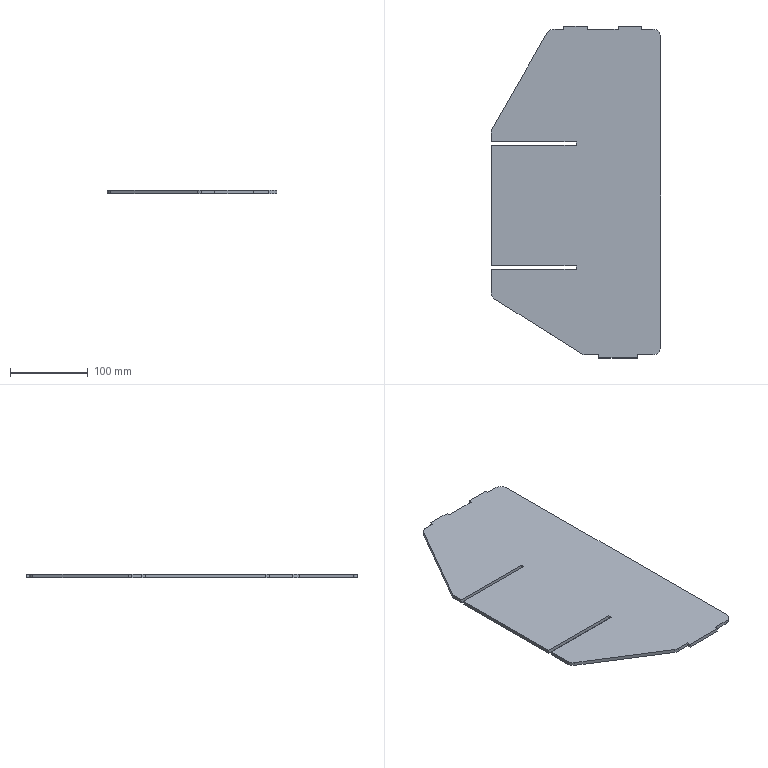Part | SolidWorks | features FlatPattern 1, SMBaseFlange 1, SheetMetal 1 | 1 solid | 34 faces | box 218.7 x 428.4 x 4.5 mm | volume 369053 mm3 | plane 28 | cylinder 6 | commonest cylinder face diameters 20 x6
STEP:
#1=CARTESIAN_POINT('',(-227.2,-382.479,0.));
#2=VERTEX_POINT('',#1);
#3=CARTESIAN_POINT('',(-227.2,-395.3,0.));
#4=VERTEX_POINT('',#3);
#5=CARTESIAN_POINT('',(-227.2,-395.3,0.));
#6=DIRECTION('',(0.,-1.,0.));
#7=VECTOR('',#6,1000.);
#8=LINE('',#5,#7);
#9=EDGE_CURVE('',#2,#4,#8,.T.);
#10=ORIENTED_EDGE('',*,*,#9,.T.);
#11=CARTESIAN_POINT('',(-227.2,-395.3,4.5));
#12=VERTEX_POINT('',#11);
#13=CARTESIAN_POINT('',(-227.2,-395.3,4.5));
#14=DIRECTION('',(0.,0.,-1.));
#15=VECTOR('',#14,1000.);
#16=LINE('',#13,#15);
#17=EDGE_CURVE('',#12,#4,#16,.T.);
#18=ORIENTED_EDGE('',*,*,#17,.F.);
#19=CARTESIAN_POINT('',(-227.2,-382.479,4.5));
#20=VERTEX_POINT('',#19);
#21=CARTESIAN_POINT('',(-227.2,-395.3,4.5));
#22=DIRECTION('',(0.,-1.,0.));
#23=VECTOR('',#22,1000.);
#24=LINE('',#21,#23);
#25=EDGE_CURVE('',#20,#12,#24,.T.);
#26=ORIENTED_EDGE('',*,*,#25,.F.);
#27=CARTESIAN_POINT('',(-227.2,-382.479,4.5));
#28=DIRECTION('',(0.,0.,-1.));
#29=VECTOR('',#28,1000.);
#30=LINE('',#27,#29);
#31=EDGE_CURVE('',#20,#2,#30,.T.);
#32=ORIENTED_EDGE('',*,*,#31,.T.);
#33=EDGE_LOOP('',(#10,#18,#26,#32));
#34=FACE_OUTER_BOUND('',#33,.T.);
#35=CARTESIAN_POINT('',(-227.2,-395.3,4.5));
#36=DIRECTION('',(1.,0.,0.));
#37=DIRECTION('',(0.,0.,-1.));
#38=AXIS2_PLACEMENT_3D('',#35,#36,#37);
#39=PLANE('',#38);
#40=ADVANCED_FACE('',(#34),#39,.F.);
#41=CARTESIAN_POINT('',(-117.7,-395.3,0.));
#42=VERTEX_POINT('',#41);
#43=CARTESIAN_POINT('',(-227.2,-395.3,0.));
#44=DIRECTION('',(1.,0.,0.));
#45=VECTOR('',#44,1000.);
#46=LINE('',#43,#45);
#47=EDGE_CURVE('',#4,#42,#46,.T.);
#48=ORIENTED_EDGE('',*,*,#47,.T.);
#49=CARTESIAN_POINT('',(-117.7,-395.3,4.5));
#50=VERTEX_POINT('',#49);
#51=CARTESIAN_POINT('',(-117.7,-395.3,4.5));
#52=DIRECTION('',(0.,0.,-1.));
#53=VECTOR('',#52,1000.);
#54=LINE('',#51,#53);
#55=EDGE_CURVE('',#50,#42,#54,.T.);
#56=ORIENTED_EDGE('',*,*,#55,.F.);
#57=CARTESIAN_POINT('',(-227.2,-395.3,4.5));
#58=DIRECTION('',(1.,0.,0.));
#59=VECTOR('',#58,1000.);
#60=LINE('',#57,#59);
#61=EDGE_CURVE('',#12,#50,#60,.T.);
#62=ORIENTED_EDGE('',*,*,#61,.F.);
#63=ORIENTED_EDGE('',*,*,#17,.T.);
#64=EDGE_LOOP('',(#48,#56,#62,#63));
#65=FACE_OUTER_BOUND('',#64,.T.);
#66=CARTESIAN_POINT('',(-227.2,-395.3,4.5));
#67=DIRECTION('',(0.,1.,0.));
#68=DIRECTION('',(-1.,0.,0.));
#69=AXIS2_PLACEMENT_3D('',#66,#67,#68);
#70=PLANE('',#69);
#71=ADVANCED_FACE('',(#65),#70,.F.);
#72=CARTESIAN_POINT('',(-117.7,-399.8,0.));
#73=VERTEX_POINT('',#72);
#74=CARTESIAN_POINT('',(-117.7,-395.3,0.));
#75=DIRECTION('',(0.,-1.,0.));
#76=VECTOR('',#75,1000.);
#77=LINE('',#74,#76);
#78=EDGE_CURVE('',#42,#73,#77,.T.);
#79=ORIENTED_EDGE('',*,*,#78,.T.);
#80=CARTESIAN_POINT('',(-117.7,-399.8,4.5));
#81=VERTEX_POINT('',#80);
#82=CARTESIAN_POINT('',(-117.7,-399.8,4.5));
#83=DIRECTION('',(0.,0.,-1.));
#84=VECTOR('',#83,1000.);
#85=LINE('',#82,#84);
#86=EDGE_CURVE('',#81,#73,#85,.T.);
#87=ORIENTED_EDGE('',*,*,#86,.F.);
#88=CARTESIAN_POINT('',(-117.7,-395.3,4.5));
#89=DIRECTION('',(0.,-1.,0.));
#90=VECTOR('',#89,1000.);
#91=LINE('',#88,#90);
#92=EDGE_CURVE('',#50,#81,#91,.T.);
#93=ORIENTED_EDGE('',*,*,#92,.F.);
#94=ORIENTED_EDGE('',*,*,#55,.T.);
#95=EDGE_LOOP('',(#79,#87,#93,#94));
#96=FACE_OUTER_BOUND('',#95,.T.);
#97=CARTESIAN_POINT('',(-117.7,-395.3,4.5));
#98=DIRECTION('',(1.,0.,0.));
#99=DIRECTION('',(0.,0.,-1.));
#100=AXIS2_PLACEMENT_3D('',#97,#98,#99);
#101=PLANE('',#100);
#102=ADVANCED_FACE('',(#96),#101,.F.);
#103=CARTESIAN_POINT('',(-227.2,-399.8,0.));
#104=VERTEX_POINT('',#103);
#105=CARTESIAN_POINT('',(-117.7,-399.8,0.));
#106=DIRECTION('',(-1.,0.,0.));
#107=VECTOR('',#106,1000.);
#108=LINE('',#105,#107);
#109=EDGE_CURVE('',#73,#104,#108,.T.);
#110=ORIENTED_EDGE('',*,*,#109,.T.);
#111=CARTESIAN_POINT('',(-227.2,-399.8,4.5));
#112=VERTEX_POINT('',#111);
#113=CARTESIAN_POINT('',(-227.2,-399.8,4.5));
#114=DIRECTION('',(0.,0.,-1.));
#115=VECTOR('',#114,1000.);
#116=LINE('',#113,#115);
#117=EDGE_CURVE('',#112,#104,#116,.T.);
#118=ORIENTED_EDGE('',*,*,#117,.F.);
#119=CARTESIAN_POINT('',(-117.7,-399.8,4.5));
#120=DIRECTION('',(-1.,0.,0.));
#121=VECTOR('',#120,1000.);
#122=LINE('',#119,#121);
#123=EDGE_CURVE('',#81,#112,#122,.T.);
#124=ORIENTED_EDGE('',*,*,#123,.F.);
#125=ORIENTED_EDGE('',*,*,#86,.T.);
#126=EDGE_LOOP('',(#110,#118,#124,#125));
#127=FACE_OUTER_BOUND('',#126,.T.);
#128=CARTESIAN_POINT('',(-117.7,-399.8,4.5));
#129=DIRECTION('',(0.,-1.,0.));
#130=DIRECTION('',(0.,0.,-1.));
#131=AXIS2_PLACEMENT_3D('',#128,#129,#130);
#132=PLANE('',#131);
#133=ADVANCED_FACE('',(#127),#132,.F.);
#134=CARTESIAN_POINT('',(-227.2,-555.3,0.));
#135=VERTEX_POINT('',#134);
#136=CARTESIAN_POINT('',(-227.2,-555.3,0.));
#137=DIRECTION('',(0.,-1.,0.));
#138=VECTOR('',#137,1000.);
#139=LINE('',#136,#138);
#140=EDGE_CURVE('',#104,#135,#139,.T.);
#141=ORIENTED_EDGE('',*,*,#140,.T.);
#142=CARTESIAN_POINT('',(-227.2,-555.3,4.5));
#143=VERTEX_POINT('',#142);
#144=CARTESIAN_POINT('',(-227.2,-555.3,4.5));
#145=DIRECTION('',(0.,0.,-1.));
#146=VECTOR('',#145,1000.);
#147=LINE('',#144,#146);
#148=EDGE_CURVE('',#143,#135,#147,.T.);
#149=ORIENTED_EDGE('',*,*,#148,.F.);
#150=CARTESIAN_POINT('',(-227.2,-555.3,4.5));
#151=DIRECTION('',(0.,-1.,0.));
#152=VECTOR('',#151,1000.);
#153=LINE('',#150,#152);
#154=EDGE_CURVE('',#112,#143,#153,.T.);
#155=ORIENTED_EDGE('',*,*,#154,.F.);
#156=ORIENTED_EDGE('',*,*,#117,.T.);
#157=EDGE_LOOP('',(#141,#149,#155,#156));
#158=FACE_OUTER_BOUND('',#157,.T.);
#159=CARTESIAN_POINT('',(-227.2,-555.3,4.5));
#160=DIRECTION('',(1.,0.,0.));
#161=DIRECTION('',(0.,0.,-1.));
#162=AXIS2_PLACEMENT_3D('',#159,#160,#161);
#163=PLANE('',#162);
#164=ADVANCED_FACE('',(#158),#163,.F.);
#165=CARTESIAN_POINT('',(-117.7,-555.3,0.));
#166=VERTEX_POINT('',#165);
#167=CARTESIAN_POINT('',(-227.2,-555.3,0.));
#168=DIRECTION('',(1.,0.,0.));
#169=VECTOR('',#168,1000.);
#170=LINE('',#167,#169);
#171=EDGE_CURVE('',#135,#166,#170,.T.);
#172=ORIENTED_EDGE('',*,*,#171,.T.);
#173=CARTESIAN_POINT('',(-117.7,-555.3,4.5));
#174=VERTEX_POINT('',#173);
#175=CARTESIAN_POINT('',(-117.7,-555.3,4.5));
#176=DIRECTION('',(0.,0.,-1.));
#177=VECTOR('',#176,1000.);
#178=LINE('',#175,#177);
#179=EDGE_CURVE('',#174,#166,#178,.T.);
#180=ORIENTED_EDGE('',*,*,#179,.F.);
#181=CARTESIAN_POINT('',(-227.2,-555.3,4.5));
#182=DIRECTION('',(1.,0.,0.));
#183=VECTOR('',#182,1000.);
#184=LINE('',#181,#183);
#185=EDGE_CURVE('',#143,#174,#184,.T.);
#186=ORIENTED_EDGE('',*,*,#185,.F.);
#187=ORIENTED_EDGE('',*,*,#148,.T.);
#188=EDGE_LOOP('',(#172,#180,#186,#187));
#189=FACE_OUTER_BOUND('',#188,.T.);
#190=CARTESIAN_POINT('',(-227.2,-555.3,4.5));
#191=DIRECTION('',(0.,1.,0.));
#192=DIRECTION('',(-1.,0.,0.));
#193=AXIS2_PLACEMENT_3D('',#190,#191,#192);
#194=PLANE('',#193);
#195=ADVANCED_FACE('',(#189),#194,.F.);
#196=CARTESIAN_POINT('',(-117.7,-559.8,0.));
#197=VERTEX_POINT('',#196);
#198=CARTESIAN_POINT('',(-117.7,-555.3,0.));
#199=DIRECTION('',(0.,-1.,0.));
#200=VECTOR('',#199,1000.);
#201=LINE('',#198,#200);
#202=EDGE_CURVE('',#166,#197,#201,.T.);
#203=ORIENTED_EDGE('',*,*,#202,.T.);
#204=CARTESIAN_POINT('',(-117.7,-559.8,4.5));
#205=VERTEX_POINT('',#204);
#206=CARTESIAN_POINT('',(-117.7,-559.8,4.5));
#207=DIRECTION('',(0.,0.,-1.));
#208=VECTOR('',#207,1000.);
#209=LINE('',#206,#208);
#210=EDGE_CURVE('',#205,#197,#209,.T.);
#211=ORIENTED_EDGE('',*,*,#210,.F.);
#212=CARTESIAN_POINT('',(-117.7,-555.3,4.5));
#213=DIRECTION('',(0.,-1.,0.));
#214=VECTOR('',#213,1000.);
#215=LINE('',#212,#214);
#216=EDGE_CURVE('',#174,#205,#215,.T.);
#217=ORIENTED_EDGE('',*,*,#216,.F.);
#218=ORIENTED_EDGE('',*,*,#179,.T.);
#219=EDGE_LOOP('',(#203,#211,#217,#218));
#220=FACE_OUTER_BOUND('',#219,.T.);
#221=CARTESIAN_POINT('',(-117.7,-555.3,4.5));
#222=DIRECTION('',(1.,0.,0.));
#223=DIRECTION('',(0.,1.,0.));
#224=AXIS2_PLACEMENT_3D('',#221,#222,#223);
#225=PLANE('',#224);
#226=ADVANCED_FACE('',(#220),#225,.F.);
#227=CARTESIAN_POINT('',(-227.2,-559.8,0.));
#228=VERTEX_POINT('',#227);
#229=CARTESIAN_POINT('',(-117.7,-559.8,0.));
#230=DIRECTION('',(-1.,0.,0.));
#231=VECTOR('',#230,1000.);
#232=LINE('',#229,#231);
#233=EDGE_CURVE('',#197,#228,#232,.T.);
#234=ORIENTED_EDGE('',*,*,#233,.T.);
#235=CARTESIAN_POINT('',(-227.2,-559.8,4.5));
#236=VERTEX_POINT('',#235);
#237=CARTESIAN_POINT('',(-227.2,-559.8,4.5));
#238=DIRECTION('',(0.,0.,-1.));
#239=VECTOR('',#238,1000.);
#240=LINE('',#237,#239);
#241=EDGE_CURVE('',#236,#228,#240,.T.);
#242=ORIENTED_EDGE('',*,*,#241,.F.);
#243=CARTESIAN_POINT('',(-117.7,-559.8,4.5));
#244=DIRECTION('',(-1.,0.,0.));
#245=VECTOR('',#244,1000.);
#246=LINE('',#243,#245);
#247=EDGE_CURVE('',#205,#236,#246,.T.);
#248=ORIENTED_EDGE('',*,*,#247,.F.);
#249=ORIENTED_EDGE('',*,*,#210,.T.);
#250=EDGE_LOOP('',(#234,#242,#248,#249));
#251=FACE_OUTER_BOUND('',#250,.T.);
#252=CARTESIAN_POINT('',(-117.7,-559.8,4.5));
#253=DIRECTION('',(0.,-1.,0.));
#254=DIRECTION('',(0.,0.,-1.));
#255=AXIS2_PLACEMENT_3D('',#252,#253,#254);
#256=PLANE('',#255);
#257=ADVANCED_FACE('',(#251),#256,.F.);
#258=CARTESIAN_POINT('',(-227.2,-589.69,0.));
#259=VERTEX_POINT('',#258);
#260=CARTESIAN_POINT('',(-227.2,-589.69,0.));
#261=DIRECTION('',(0.,-1.,0.));
#262=VECTOR('',#261,1000.);
#263=LINE('',#260,#262);
#264=EDGE_CURVE('',#228,#259,#263,.T.);
#265=ORIENTED_EDGE('',*,*,#264,.T.);
#266=CARTESIAN_POINT('',(-227.2,-589.69,4.5));
#267=VERTEX_POINT('',#266);
#268=CARTESIAN_POINT('',(-227.2,-589.69,4.5));
#269=DIRECTION('',(0.,0.,-1.));
#270=VECTOR('',#269,1000.);
#271=LINE('',#268,#270);
#272=EDGE_CURVE('',#267,#259,#271,.T.);
#273=ORIENTED_EDGE('',*,*,#272,.F.);
#274=CARTESIAN_POINT('',(-227.2,-589.69,4.5));
#275=DIRECTION('',(0.,-1.,0.));
#276=VECTOR('',#275,1000.);
#277=LINE('',#274,#276);
#278=EDGE_CURVE('',#236,#267,#277,.T.);
#279=ORIENTED_EDGE('',*,*,#278,.F.);
#280=ORIENTED_EDGE('',*,*,#241,.T.);
#281=EDGE_LOOP('',(#265,#273,#279,#280));
#282=FACE_OUTER_BOUND('',#281,.T.);
#283=CARTESIAN_POINT('',(-227.2,-589.69,4.5));
#284=DIRECTION('',(1.,0.,0.));
#285=DIRECTION('',(0.,0.,-1.));
#286=AXIS2_PLACEMENT_3D('',#283,#284,#285);
#287=PLANE('',#286);
#288=ADVANCED_FACE('',(#282),#287,.F.);
#289=CARTESIAN_POINT('',(-222.541,-598.143,0.));
#290=VERTEX_POINT('',#289);
#291=CARTESIAN_POINT('',(-217.2,-589.69,0.));
#292=DIRECTION('',(0.,0.,1.));
#293=DIRECTION('',(-1.,0.,0.));
#294=AXIS2_PLACEMENT_3D('',#291,#292,#293);
#295=CIRCLE('',#294,10.);
#296=EDGE_CURVE('',#259,#290,#295,.T.);
#297=ORIENTED_EDGE('',*,*,#296,.T.);
#298=CARTESIAN_POINT('',(-222.541,-598.143,4.5));
#299=VERTEX_POINT('',#298);
#300=CARTESIAN_POINT('',(-222.541,-598.143,4.5));
#301=DIRECTION('',(0.,0.,-1.));
#302=VECTOR('',#301,1000.);
#303=LINE('',#300,#302);
#304=EDGE_CURVE('',#299,#290,#303,.T.);
#305=ORIENTED_EDGE('',*,*,#304,.F.);
#306=CARTESIAN_POINT('',(-217.2,-589.69,4.5));
#307=DIRECTION('',(0.,0.,1.));
#308=DIRECTION('',(-1.,0.,0.));
#309=AXIS2_PLACEMENT_3D('',#306,#307,#308);
#310=CIRCLE('',#309,10.);
#311=EDGE_CURVE('',#267,#299,#310,.T.);
#312=ORIENTED_EDGE('',*,*,#311,.F.);
#313=ORIENTED_EDGE('',*,*,#272,.T.);
#314=EDGE_LOOP('',(#297,#305,#312,#313));
#315=FACE_OUTER_BOUND('',#314,.T.);
#316=CARTESIAN_POINT('',(-217.2,-589.69,4.5));
#317=DIRECTION('',(0.,0.,-1.));
#318=DIRECTION('',(-1.,0.,0.));
#319=AXIS2_PLACEMENT_3D('',#316,#317,#318);
#320=CYLINDRICAL_SURFACE('',#319,10.);
#321=ADVANCED_FACE('',(#315),#320,.T.);
#322=CARTESIAN_POINT('',(-110.947,-668.654,0.));
#323=VERTEX_POINT('',#322);
#324=CARTESIAN_POINT('',(-222.541,-598.143,0.));
#325=DIRECTION('',(0.8454,-0.5342,0.));
#326=VECTOR('',#325,1000.);
#327=LINE('',#324,#326);
#328=EDGE_CURVE('',#290,#323,#327,.T.);
#329=ORIENTED_EDGE('',*,*,#328,.T.);
#330=CARTESIAN_POINT('',(-110.947,-668.654,4.5));
#331=VERTEX_POINT('',#330);
#332=CARTESIAN_POINT('',(-110.947,-668.654,4.5));
#333=DIRECTION('',(0.,0.,-1.));
#334=VECTOR('',#333,1000.);
#335=LINE('',#332,#334);
#336=EDGE_CURVE('',#331,#323,#335,.T.);
#337=ORIENTED_EDGE('',*,*,#336,.F.);
#338=CARTESIAN_POINT('',(-222.541,-598.143,4.5));
#339=DIRECTION('',(0.8454,-0.5342,0.));
#340=VECTOR('',#339,1000.);
#341=LINE('',#338,#340);
#342=EDGE_CURVE('',#299,#331,#341,.T.);
#343=ORIENTED_EDGE('',*,*,#342,.F.);
#344=ORIENTED_EDGE('',*,*,#304,.T.);
#345=EDGE_LOOP('',(#329,#337,#343,#344));
#346=FACE_OUTER_BOUND('',#345,.T.);
#347=CARTESIAN_POINT('',(-222.541,-598.143,4.5));
#348=DIRECTION('',(0.5342,0.8454,0.));
#349=DIRECTION('',(-0.8454,0.5342,0.));
#350=AXIS2_PLACEMENT_3D('',#347,#348,#349);
#351=PLANE('',#350);
#352=ADVANCED_FACE('',(#346),#351,.F.);
#353=CARTESIAN_POINT('',(-105.605,-670.2,0.));
#354=VERTEX_POINT('',#353);
#355=CARTESIAN_POINT('',(-105.605,-660.2,0.));
#356=DIRECTION('',(0.,0.,1.));
#357=DIRECTION('',(-1.,0.,0.));
#358=AXIS2_PLACEMENT_3D('',#355,#356,#357);
#359=CIRCLE('',#358,10.);
#360=EDGE_CURVE('',#323,#354,#359,.T.);
#361=ORIENTED_EDGE('',*,*,#360,.T.);
#362=CARTESIAN_POINT('',(-105.605,-670.2,4.5));
#363=VERTEX_POINT('',#362);
#364=CARTESIAN_POINT('',(-105.605,-670.2,4.5));
#365=DIRECTION('',(0.,0.,-1.));
#366=VECTOR('',#365,1000.);
#367=LINE('',#364,#366);
#368=EDGE_CURVE('',#363,#354,#367,.T.);
#369=ORIENTED_EDGE('',*,*,#368,.F.);
#370=CARTESIAN_POINT('',(-105.605,-660.2,4.5));
#371=DIRECTION('',(0.,0.,1.));
#372=DIRECTION('',(-1.,0.,0.));
#373=AXIS2_PLACEMENT_3D('',#370,#371,#372);
#374=CIRCLE('',#373,10.);
#375=EDGE_CURVE('',#331,#363,#374,.T.);
#376=ORIENTED_EDGE('',*,*,#375,.F.);
#377=ORIENTED_EDGE('',*,*,#336,.T.);
#378=EDGE_LOOP('',(#361,#369,#376,#377));
#379=FACE_OUTER_BOUND('',#378,.T.);
#380=CARTESIAN_POINT('',(-105.605,-660.2,4.5));
#381=DIRECTION('',(0.,0.,-1.));
#382=DIRECTION('',(-1.,0.,0.));
#383=AXIS2_PLACEMENT_3D('',#380,#381,#382);
#384=CYLINDRICAL_SURFACE('',#383,10.);
#385=ADVANCED_FACE('',(#379),#384,.T.);
#386=CARTESIAN_POINT('',(-88.5,-670.2,0.));
#387=VERTEX_POINT('',#386);
#388=CARTESIAN_POINT('',(-105.605,-670.2,0.));
#389=DIRECTION('',(1.,0.,0.));
#390=VECTOR('',#389,1000.);
#391=LINE('',#388,#390);
#392=EDGE_CURVE('',#354,#387,#391,.T.);
#393=ORIENTED_EDGE('',*,*,#392,.T.);
#394=CARTESIAN_POINT('',(-88.5,-670.2,4.5));
#395=VERTEX_POINT('',#394);
#396=CARTESIAN_POINT('',(-88.5,-670.2,4.5));
#397=DIRECTION('',(0.,0.,-1.));
#398=VECTOR('',#397,1000.);
#399=LINE('',#396,#398);
#400=EDGE_CURVE('',#395,#387,#399,.T.);
#401=ORIENTED_EDGE('',*,*,#400,.F.);
#402=CARTESIAN_POINT('',(-105.605,-670.2,4.5));
#403=DIRECTION('',(1.,0.,0.));
#404=VECTOR('',#403,1000.);
#405=LINE('',#402,#404);
#406=EDGE_CURVE('',#363,#395,#405,.T.);
#407=ORIENTED_EDGE('',*,*,#406,.F.);
#408=ORIENTED_EDGE('',*,*,#368,.T.);
#409=EDGE_LOOP('',(#393,#401,#407,#408));
#410=FACE_OUTER_BOUND('',#409,.T.);
#411=CARTESIAN_POINT('',(-105.605,-670.2,4.5));
#412=DIRECTION('',(0.,1.,0.));
#413=DIRECTION('',(-1.,0.,0.));
#414=AXIS2_PLACEMENT_3D('',#411,#412,#413);
#415=PLANE('',#414);
#416=ADVANCED_FACE('',(#410),#415,.F.);
#417=CARTESIAN_POINT('',(-88.5,-674.2,0.));
#418=VERTEX_POINT('',#417);
#419=CARTESIAN_POINT('',(-88.5,-674.2,0.));
#420=DIRECTION('',(0.,-1.,0.));
#421=VECTOR('',#420,1000.);
#422=LINE('',#419,#421);
#423=EDGE_CURVE('',#387,#418,#422,.T.);
#424=ORIENTED_EDGE('',*,*,#423,.T.);
#425=CARTESIAN_POINT('',(-88.5,-674.2,4.5));
#426=VERTEX_POINT('',#425);
#427=CARTESIAN_POINT('',(-88.5,-674.2,4.5));
#428=DIRECTION('',(0.,0.,-1.));
#429=VECTOR('',#428,1000.);
#430=LINE('',#427,#429);
#431=EDGE_CURVE('',#426,#418,#430,.T.);
#432=ORIENTED_EDGE('',*,*,#431,.F.);
#433=CARTESIAN_POINT('',(-88.5,-674.2,4.5));
#434=DIRECTION('',(0.,-1.,0.));
#435=VECTOR('',#434,1000.);
#436=LINE('',#433,#435);
#437=EDGE_CURVE('',#395,#426,#436,.T.);
#438=ORIENTED_EDGE('',*,*,#437,.F.);
#439=ORIENTED_EDGE('',*,*,#400,.T.);
#440=EDGE_LOOP('',(#424,#432,#438,#439));
#441=FACE_OUTER_BOUND('',#440,.T.);
#442=CARTESIAN_POINT('',(-88.5,-674.2,4.5));
#443=DIRECTION('',(1.,0.,0.));
#444=DIRECTION('',(0.,0.,-1.));
#445=AXIS2_PLACEMENT_3D('',#442,#443,#444);
#446=PLANE('',#445);
#447=ADVANCED_FACE('',(#441),#446,.F.);
#448=CARTESIAN_POINT('',(-38.5,-674.2,0.));
#449=VERTEX_POINT('',#448);
#450=CARTESIAN_POINT('',(-38.5,-674.2,0.));
#451=DIRECTION('',(1.,0.,0.));
#452=VECTOR('',#451,1000.);
#453=LINE('',#450,#452);
#454=EDGE_CURVE('',#418,#449,#453,.T.);
#455=ORIENTED_EDGE('',*,*,#454,.T.);
#456=CARTESIAN_POINT('',(-38.5,-674.2,4.5));
#457=VERTEX_POINT('',#456);
#458=CARTESIAN_POINT('',(-38.5,-674.2,4.5));
#459=DIRECTION('',(0.,0.,-1.));
#460=VECTOR('',#459,1000.);
#461=LINE('',#458,#460);
#462=EDGE_CURVE('',#457,#449,#461,.T.);
#463=ORIENTED_EDGE('',*,*,#462,.F.);
#464=CARTESIAN_POINT('',(-38.5,-674.2,4.5));
#465=DIRECTION('',(1.,0.,0.));
#466=VECTOR('',#465,1000.);
#467=LINE('',#464,#466);
#468=EDGE_CURVE('',#426,#457,#467,.T.);
#469=ORIENTED_EDGE('',*,*,#468,.F.);
#470=ORIENTED_EDGE('',*,*,#431,.T.);
#471=EDGE_LOOP('',(#455,#463,#469,#470));
#472=FACE_OUTER_BOUND('',#471,.T.);
#473=CARTESIAN_POINT('',(-38.5,-674.2,4.5));
#474=DIRECTION('',(0.,1.,0.));
#475=DIRECTION('',(0.,0.,1.));
#476=AXIS2_PLACEMENT_3D('',#473,#474,#475);
#477=PLANE('',#476);
#478=ADVANCED_FACE('',(#472),#477,.F.);
#479=CARTESIAN_POINT('',(-38.5,-670.2,0.));
#480=VERTEX_POINT('',#479);
#481=CARTESIAN_POINT('',(-38.5,-670.2,0.));
#482=DIRECTION('',(0.,1.,0.));
#483=VECTOR('',#482,1000.);
#484=LINE('',#481,#483);
#485=EDGE_CURVE('',#449,#480,#484,.T.);
#486=ORIENTED_EDGE('',*,*,#485,.T.);
#487=CARTESIAN_POINT('',(-38.5,-670.2,4.5));
#488=VERTEX_POINT('',#487);
#489=CARTESIAN_POINT('',(-38.5,-670.2,4.5));
#490=DIRECTION('',(0.,0.,-1.));
#491=VECTOR('',#490,1000.);
#492=LINE('',#489,#491);
#493=EDGE_CURVE('',#488,#480,#492,.T.);
#494=ORIENTED_EDGE('',*,*,#493,.F.);
#495=CARTESIAN_POINT('',(-38.5,-670.2,4.5));
#496=DIRECTION('',(0.,1.,0.));
#497=VECTOR('',#496,1000.);
#498=LINE('',#495,#497);
#499=EDGE_CURVE('',#457,#488,#498,.T.);
#500=ORIENTED_EDGE('',*,*,#499,.F.);
#501=ORIENTED_EDGE('',*,*,#462,.T.);
#502=EDGE_LOOP('',(#486,#494,#500,#501));
#503=FACE_OUTER_BOUND('',#502,.T.);
#504=CARTESIAN_POINT('',(-38.5,-670.2,4.5));
#505=DIRECTION('',(-1.,0.,0.));
#506=DIRECTION('',(0.,-1.,0.));
#507=AXIS2_PLACEMENT_3D('',#504,#505,#506);
#508=PLANE('',#507);
#509=ADVANCED_FACE('',(#503),#508,.F.);
#510=CARTESIAN_POINT('',(-18.5,-670.2,0.));
#511=VERTEX_POINT('',#510);
#512=CARTESIAN_POINT('',(-18.5,-670.2,0.));
#513=DIRECTION('',(1.,0.,0.));
#514=VECTOR('',#513,1000.);
#515=LINE('',#512,#514);
#516=EDGE_CURVE('',#480,#511,#515,.T.);
#517=ORIENTED_EDGE('',*,*,#516,.T.);
#518=CARTESIAN_POINT('',(-18.5,-670.2,4.5));
#519=VERTEX_POINT('',#518);
#520=CARTESIAN_POINT('',(-18.5,-670.2,4.5));
#521=DIRECTION('',(0.,0.,-1.));
#522=VECTOR('',#521,1000.);
#523=LINE('',#520,#522);
#524=EDGE_CURVE('',#519,#511,#523,.T.);
#525=ORIENTED_EDGE('',*,*,#524,.F.);
#526=CARTESIAN_POINT('',(-18.5,-670.2,4.5));
#527=DIRECTION('',(1.,0.,0.));
#528=VECTOR('',#527,1000.);
#529=LINE('',#526,#528);
#530=EDGE_CURVE('',#488,#519,#529,.T.);
#531=ORIENTED_EDGE('',*,*,#530,.F.);
#532=ORIENTED_EDGE('',*,*,#493,.T.);
#533=EDGE_LOOP('',(#517,#525,#531,#532));
#534=FACE_OUTER_BOUND('',#533,.T.);
#535=CARTESIAN_POINT('',(-18.5,-670.2,4.5));
#536=DIRECTION('',(0.,1.,0.));
#537=DIRECTION('',(-1.,0.,0.));
#538=AXIS2_PLACEMENT_3D('',#535,#536,#537);
#539=PLANE('',#538);
#540=ADVANCED_FACE('',(#534),#539,.F.);
#541=CARTESIAN_POINT('',(-8.5,-660.2,0.));
#542=VERTEX_POINT('',#541);
#543=CARTESIAN_POINT('',(-18.5,-660.2,0.));
#544=DIRECTION('',(0.,0.,1.));
#545=DIRECTION('',(-1.,0.,0.));
#546=AXIS2_PLACEMENT_3D('',#543,#544,#545);
#547=CIRCLE('',#546,10.);
#548=EDGE_CURVE('',#511,#542,#547,.T.);
#549=ORIENTED_EDGE('',*,*,#548,.T.);
#550=CARTESIAN_POINT('',(-8.5,-660.2,4.5));
#551=VERTEX_POINT('',#550);
#552=CARTESIAN_POINT('',(-8.5,-660.2,4.5));
#553=DIRECTION('',(0.,0.,-1.));
#554=VECTOR('',#553,1000.);
#555=LINE('',#552,#554);
#556=EDGE_CURVE('',#551,#542,#555,.T.);
#557=ORIENTED_EDGE('',*,*,#556,.F.);
#558=CARTESIAN_POINT('',(-18.5,-660.2,4.5));
#559=DIRECTION('',(0.,0.,1.));
#560=DIRECTION('',(-1.,0.,0.));
#561=AXIS2_PLACEMENT_3D('',#558,#559,#560);
#562=CIRCLE('',#561,10.);
#563=EDGE_CURVE('',#519,#551,#562,.T.);
#564=ORIENTED_EDGE('',*,*,#563,.F.);
#565=ORIENTED_EDGE('',*,*,#524,.T.);
#566=EDGE_LOOP('',(#549,#557,#564,#565));
#567=FACE_OUTER_BOUND('',#566,.T.);
#568=CARTESIAN_POINT('',(-18.5,-660.2,4.5));
#569=DIRECTION('',(0.,0.,-1.));
#570=DIRECTION('',(-1.,0.,0.));
#571=AXIS2_PLACEMENT_3D('',#568,#569,#570);
#572=CYLINDRICAL_SURFACE('',#571,10.);
#573=ADVANCED_FACE('',(#567),#572,.T.);
#574=CARTESIAN_POINT('',(-8.5,-259.8,0.));
#575=VERTEX_POINT('',#574);
#576=CARTESIAN_POINT('',(-8.5,-259.8,0.));
#577=DIRECTION('',(0.,1.,0.));
#578=VECTOR('',#577,1000.);
#579=LINE('',#576,#578);
#580=EDGE_CURVE('',#542,#575,#579,.T.);
#581=ORIENTED_EDGE('',*,*,#580,.T.);
#582=CARTESIAN_POINT('',(-8.5,-259.8,4.5));
#583=VERTEX_POINT('',#582);
#584=CARTESIAN_POINT('',(-8.5,-259.8,4.5));
#585=DIRECTION('',(0.,0.,-1.));
#586=VECTOR('',#585,1000.);
#587=LINE('',#584,#586);
#588=EDGE_CURVE('',#583,#575,#587,.T.);
#589=ORIENTED_EDGE('',*,*,#588,.F.);
#590=CARTESIAN_POINT('',(-8.5,-259.8,4.5));
#591=DIRECTION('',(0.,1.,0.));
#592=VECTOR('',#591,1000.);
#593=LINE('',#590,#592);
#594=EDGE_CURVE('',#551,#583,#593,.T.);
#595=ORIENTED_EDGE('',*,*,#594,.F.);
#596=ORIENTED_EDGE('',*,*,#556,.T.);
#597=EDGE_LOOP('',(#581,#589,#595,#596));
#598=FACE_OUTER_BOUND('',#597,.T.);
#599=CARTESIAN_POINT('',(-8.5,-259.8,4.5));
#600=DIRECTION('',(-1.,0.,0.));
#601=DIRECTION('',(0.,-1.,0.));
#602=AXIS2_PLACEMENT_3D('',#599,#600,#601);
#603=PLANE('',#602);
#604=ADVANCED_FACE('',(#598),#603,.F.);
#605=CARTESIAN_POINT('',(-18.5,-249.8,0.));
#606=VERTEX_POINT('',#605);
#607=CARTESIAN_POINT('',(-18.5,-259.8,0.));
#608=DIRECTION('',(0.,0.,1.));
#609=DIRECTION('',(1.,0.,0.));
#610=AXIS2_PLACEMENT_3D('',#607,#608,#609);
#611=CIRCLE('',#610,10.);
#612=EDGE_CURVE('',#575,#606,#611,.T.);
#613=ORIENTED_EDGE('',*,*,#612,.T.);
#614=CARTESIAN_POINT('',(-18.5,-249.8,4.5));
#615=VERTEX_POINT('',#614);
#616=CARTESIAN_POINT('',(-18.5,-249.8,4.5));
#617=DIRECTION('',(0.,0.,-1.));
#618=VECTOR('',#617,1000.);
#619=LINE('',#616,#618);
#620=EDGE_CURVE('',#615,#606,#619,.T.);
#621=ORIENTED_EDGE('',*,*,#620,.F.);
#622=CARTESIAN_POINT('',(-18.5,-259.8,4.5));
#623=DIRECTION('',(0.,0.,1.));
#624=DIRECTION('',(1.,0.,0.));
#625=AXIS2_PLACEMENT_3D('',#622,#623,#624);
#626=CIRCLE('',#625,10.);
#627=EDGE_CURVE('',#583,#615,#626,.T.);
#628=ORIENTED_EDGE('',*,*,#627,.F.);
#629=ORIENTED_EDGE('',*,*,#588,.T.);
#630=EDGE_LOOP('',(#613,#621,#628,#629));
#631=FACE_OUTER_BOUND('',#630,.T.);
#632=CARTESIAN_POINT('',(-18.5,-259.8,4.5));
#633=DIRECTION('',(0.,0.,-1.));
#634=DIRECTION('',(-1.,0.,0.));
#635=AXIS2_PLACEMENT_3D('',#632,#633,#634);
#636=CYLINDRICAL_SURFACE('',#635,10.);
#637=ADVANCED_FACE('',(#631),#636,.T.);
#638=CARTESIAN_POINT('',(-33.5,-249.8,0.));
#639=VERTEX_POINT('',#638);
#640=CARTESIAN_POINT('',(-18.5,-249.8,0.));
#641=DIRECTION('',(-1.,0.,0.));
#642=VECTOR('',#641,1000.);
#643=LINE('',#640,#642);
#644=EDGE_CURVE('',#606,#639,#643,.T.);
#645=ORIENTED_EDGE('',*,*,#644,.T.);
#646=CARTESIAN_POINT('',(-33.5,-249.8,4.5));
#647=VERTEX_POINT('',#646);
#648=CARTESIAN_POINT('',(-33.5,-249.8,4.5));
#649=DIRECTION('',(0.,0.,-1.));
#650=VECTOR('',#649,1000.);
#651=LINE('',#648,#650);
#652=EDGE_CURVE('',#647,#639,#651,.T.);
#653=ORIENTED_EDGE('',*,*,#652,.F.);
#654=CARTESIAN_POINT('',(-18.5,-249.8,4.5));
#655=DIRECTION('',(-1.,0.,0.));
#656=VECTOR('',#655,1000.);
#657=LINE('',#654,#656);
#658=EDGE_CURVE('',#615,#647,#657,.T.);
#659=ORIENTED_EDGE('',*,*,#658,.F.);
#660=ORIENTED_EDGE('',*,*,#620,.T.);
#661=EDGE_LOOP('',(#645,#653,#659,#660));
#662=FACE_OUTER_BOUND('',#661,.T.);
#663=CARTESIAN_POINT('',(-18.5,-249.8,4.5));
#664=DIRECTION('',(0.,-1.,0.));
#665=DIRECTION('',(1.,0.,0.));
#666=AXIS2_PLACEMENT_3D('',#663,#664,#665);
#667=PLANE('',#666);
#668=ADVANCED_FACE('',(#662),#667,.F.);
#669=CARTESIAN_POINT('',(-33.5,-245.8,0.));
#670=VERTEX_POINT('',#669);
#671=CARTESIAN_POINT('',(-33.5,-249.8,0.));
#672=DIRECTION('',(0.,1.,0.));
#673=VECTOR('',#672,1000.);
#674=LINE('',#671,#673);
#675=EDGE_CURVE('',#639,#670,#674,.T.);
#676=ORIENTED_EDGE('',*,*,#675,.T.);
#677=CARTESIAN_POINT('',(-33.5,-245.8,4.5));
#678=VERTEX_POINT('',#677);
#679=CARTESIAN_POINT('',(-33.5,-245.8,4.5));
#680=DIRECTION('',(0.,0.,-1.));
#681=VECTOR('',#680,1000.);
#682=LINE('',#679,#681);
#683=EDGE_CURVE('',#678,#670,#682,.T.);
#684=ORIENTED_EDGE('',*,*,#683,.F.);
#685=CARTESIAN_POINT('',(-33.5,-249.8,4.5));
#686=DIRECTION('',(0.,1.,0.));
#687=VECTOR('',#686,1000.);
#688=LINE('',#685,#687);
#689=EDGE_CURVE('',#647,#678,#688,.T.);
#690=ORIENTED_EDGE('',*,*,#689,.F.);
#691=ORIENTED_EDGE('',*,*,#652,.T.);
#692=EDGE_LOOP('',(#676,#684,#690,#691));
#693=FACE_OUTER_BOUND('',#692,.T.);
#694=CARTESIAN_POINT('',(-33.5,-249.8,4.5));
#695=DIRECTION('',(-1.,0.,0.));
#696=DIRECTION('',(0.,0.,1.));
#697=AXIS2_PLACEMENT_3D('',#694,#695,#696);
#698=PLANE('',#697);
#699=ADVANCED_FACE('',(#693),#698,.F.);
#700=CARTESIAN_POINT('',(-63.5,-245.8,0.));
#701=VERTEX_POINT('',#700);
#702=CARTESIAN_POINT('',(-33.5,-245.8,0.));
#703=DIRECTION('',(-1.,0.,0.));
#704=VECTOR('',#703,1000.);
#705=LINE('',#702,#704);
#706=EDGE_CURVE('',#670,#701,#705,.T.);
#707=ORIENTED_EDGE('',*,*,#706,.T.);
#708=CARTESIAN_POINT('',(-63.5,-245.8,4.5));
#709=VERTEX_POINT('',#708);
#710=CARTESIAN_POINT('',(-63.5,-245.8,4.5));
#711=DIRECTION('',(0.,0.,-1.));
#712=VECTOR('',#711,1000.);
#713=LINE('',#710,#712);
#714=EDGE_CURVE('',#709,#701,#713,.T.);
#715=ORIENTED_EDGE('',*,*,#714,.F.);
#716=CARTESIAN_POINT('',(-33.5,-245.8,4.5));
#717=DIRECTION('',(-1.,0.,0.));
#718=VECTOR('',#717,1000.);
#719=LINE('',#716,#718);
#720=EDGE_CURVE('',#678,#709,#719,.T.);
#721=ORIENTED_EDGE('',*,*,#720,.F.);
#722=ORIENTED_EDGE('',*,*,#683,.T.);
#723=EDGE_LOOP('',(#707,#715,#721,#722));
#724=FACE_OUTER_BOUND('',#723,.T.);
#725=CARTESIAN_POINT('',(-33.5,-245.8,4.5));
#726=DIRECTION('',(0.,-1.,0.));
#727=DIRECTION('',(0.,0.,-1.));
#728=AXIS2_PLACEMENT_3D('',#725,#726,#727);
#729=PLANE('',#728);
#730=ADVANCED_FACE('',(#724),#729,.F.);
#731=CARTESIAN_POINT('',(-63.5,-249.8,0.));
#732=VERTEX_POINT('',#731);
#733=CARTESIAN_POINT('',(-63.5,-245.8,0.));
#734=DIRECTION('',(0.,-1.,0.));
#735=VECTOR('',#734,1000.);
#736=LINE('',#733,#735);
#737=EDGE_CURVE('',#701,#732,#736,.T.);
#738=ORIENTED_EDGE('',*,*,#737,.T.);
#739=CARTESIAN_POINT('',(-63.5,-249.8,4.5));
#740=VERTEX_POINT('',#739);
#741=CARTESIAN_POINT('',(-63.5,-249.8,4.5));
#742=DIRECTION('',(0.,0.,-1.));
#743=VECTOR('',#742,1000.);
#744=LINE('',#741,#743);
#745=EDGE_CURVE('',#740,#732,#744,.T.);
#746=ORIENTED_EDGE('',*,*,#745,.F.);
#747=CARTESIAN_POINT('',(-63.5,-245.8,4.5));
#748=DIRECTION('',(0.,-1.,0.));
#749=VECTOR('',#748,1000.);
#750=LINE('',#747,#749);
#751=EDGE_CURVE('',#709,#740,#750,.T.);
#752=ORIENTED_EDGE('',*,*,#751,.F.);
#753=ORIENTED_EDGE('',*,*,#714,.T.);
#754=EDGE_LOOP('',(#738,#746,#752,#753));
#755=FACE_OUTER_BOUND('',#754,.T.);
#756=CARTESIAN_POINT('',(-63.5,-245.8,4.5));
#757=DIRECTION('',(1.,0.,0.));
#758=DIRECTION('',(0.,0.,-1.));
#759=AXIS2_PLACEMENT_3D('',#756,#757,#758);
#760=PLANE('',#759);
#761=ADVANCED_FACE('',(#755),#760,.F.);
#762=CARTESIAN_POINT('',(-103.5,-249.8,0.));
#763=VERTEX_POINT('',#762);
#764=CARTESIAN_POINT('',(-63.5,-249.8,0.));
#765=DIRECTION('',(-1.,0.,0.));
#766=VECTOR('',#765,1000.);
#767=LINE('',#764,#766);
#768=EDGE_CURVE('',#732,#763,#767,.T.);
#769=ORIENTED_EDGE('',*,*,#768,.T.);
#770=CARTESIAN_POINT('',(-103.5,-249.8,4.5));
#771=VERTEX_POINT('',#770);
#772=CARTESIAN_POINT('',(-103.5,-249.8,4.5));
#773=DIRECTION('',(0.,0.,-1.));
#774=VECTOR('',#773,1000.);
#775=LINE('',#772,#774);
#776=EDGE_CURVE('',#771,#763,#775,.T.);
#777=ORIENTED_EDGE('',*,*,#776,.F.);
#778=CARTESIAN_POINT('',(-63.5,-249.8,4.5));
#779=DIRECTION('',(-1.,0.,0.));
#780=VECTOR('',#779,1000.);
#781=LINE('',#778,#780);
#782=EDGE_CURVE('',#740,#771,#781,.T.);
#783=ORIENTED_EDGE('',*,*,#782,.F.);
#784=ORIENTED_EDGE('',*,*,#745,.T.);
#785=EDGE_LOOP('',(#769,#777,#783,#784));
#786=FACE_OUTER_BOUND('',#785,.T.);
#787=CARTESIAN_POINT('',(-63.5,-249.8,4.5));
#788=DIRECTION('',(0.,-1.,0.));
#789=DIRECTION('',(0.,0.,-1.));
#790=AXIS2_PLACEMENT_3D('',#787,#788,#789);
#791=PLANE('',#790);
#792=ADVANCED_FACE('',(#786),#791,.F.);
#793=CARTESIAN_POINT('',(-103.5,-245.8,0.));
#794=VERTEX_POINT('',#793);
#795=CARTESIAN_POINT('',(-103.5,-249.8,0.));
#796=DIRECTION('',(0.,1.,0.));
#797=VECTOR('',#796,1000.);
#798=LINE('',#795,#797);
#799=EDGE_CURVE('',#763,#794,#798,.T.);
#800=ORIENTED_EDGE('',*,*,#799,.T.);
#801=CARTESIAN_POINT('',(-103.5,-245.8,4.5));
#802=VERTEX_POINT('',#801);
#803=CARTESIAN_POINT('',(-103.5,-245.8,4.5));
#804=DIRECTION('',(0.,0.,-1.));
#805=VECTOR('',#804,1000.);
#806=LINE('',#803,#805);
#807=EDGE_CURVE('',#802,#794,#806,.T.);
#808=ORIENTED_EDGE('',*,*,#807,.F.);
#809=CARTESIAN_POINT('',(-103.5,-249.8,4.5));
#810=DIRECTION('',(0.,1.,0.));
#811=VECTOR('',#810,1000.);
#812=LINE('',#809,#811);
#813=EDGE_CURVE('',#771,#802,#812,.T.);
#814=ORIENTED_EDGE('',*,*,#813,.F.);
#815=ORIENTED_EDGE('',*,*,#776,.T.);
#816=EDGE_LOOP('',(#800,#808,#814,#815));
#817=FACE_OUTER_BOUND('',#816,.T.);
#818=CARTESIAN_POINT('',(-103.5,-249.8,4.5));
#819=DIRECTION('',(-1.,0.,0.));
#820=DIRECTION('',(0.,0.,1.));
#821=AXIS2_PLACEMENT_3D('',#818,#819,#820);
#822=PLANE('',#821);
#823=ADVANCED_FACE('',(#817),#822,.F.);
#824=CARTESIAN_POINT('',(-133.5,-245.8,0.));
#825=VERTEX_POINT('',#824);
#826=CARTESIAN_POINT('',(-103.5,-245.8,0.));
#827=DIRECTION('',(-1.,0.,0.));
#828=VECTOR('',#827,1000.);
#829=LINE('',#826,#828);
#830=EDGE_CURVE('',#794,#825,#829,.T.);
#831=ORIENTED_EDGE('',*,*,#830,.T.);
#832=CARTESIAN_POINT('',(-133.5,-245.8,4.5));
#833=VERTEX_POINT('',#832);
#834=CARTESIAN_POINT('',(-133.5,-245.8,4.5));
#835=DIRECTION('',(0.,0.,-1.));
#836=VECTOR('',#835,1000.);
#837=LINE('',#834,#836);
#838=EDGE_CURVE('',#833,#825,#837,.T.);
#839=ORIENTED_EDGE('',*,*,#838,.F.);
#840=CARTESIAN_POINT('',(-103.5,-245.8,4.5));
#841=DIRECTION('',(-1.,0.,0.));
#842=VECTOR('',#841,1000.);
#843=LINE('',#840,#842);
#844=EDGE_CURVE('',#802,#833,#843,.T.);
#845=ORIENTED_EDGE('',*,*,#844,.F.);
#846=ORIENTED_EDGE('',*,*,#807,.T.);
#847=EDGE_LOOP('',(#831,#839,#845,#846));
#848=FACE_OUTER_BOUND('',#847,.T.);
#849=CARTESIAN_POINT('',(-103.5,-245.8,4.5));
#850=DIRECTION('',(0.,-1.,0.));
#851=DIRECTION('',(1.,0.,0.));
#852=AXIS2_PLACEMENT_3D('',#849,#850,#851);
#853=PLANE('',#852);
#854=ADVANCED_FACE('',(#848),#853,.F.);
#855=CARTESIAN_POINT('',(-133.5,-249.8,0.));
#856=VERTEX_POINT('',#855);
#857=CARTESIAN_POINT('',(-133.5,-245.8,0.));
#858=DIRECTION('',(0.,-1.,0.));
#859=VECTOR('',#858,1000.);
#860=LINE('',#857,#859);
#861=EDGE_CURVE('',#825,#856,#860,.T.);
#862=ORIENTED_EDGE('',*,*,#861,.T.);
#863=CARTESIAN_POINT('',(-133.5,-249.8,4.5));
#864=VERTEX_POINT('',#863);
#865=CARTESIAN_POINT('',(-133.5,-249.8,4.5));
#866=DIRECTION('',(0.,0.,-1.));
#867=VECTOR('',#866,1000.);
#868=LINE('',#865,#867);
#869=EDGE_CURVE('',#864,#856,#868,.T.);
#870=ORIENTED_EDGE('',*,*,#869,.F.);
#871=CARTESIAN_POINT('',(-133.5,-245.8,4.5));
#872=DIRECTION('',(0.,-1.,0.));
#873=VECTOR('',#872,1000.);
#874=LINE('',#871,#873);
#875=EDGE_CURVE('',#833,#864,#874,.T.);
#876=ORIENTED_EDGE('',*,*,#875,.F.);
#877=ORIENTED_EDGE('',*,*,#838,.T.);
#878=EDGE_LOOP('',(#862,#870,#876,#877));
#879=FACE_OUTER_BOUND('',#878,.T.);
#880=CARTESIAN_POINT('',(-133.5,-245.8,4.5));
#881=DIRECTION('',(1.,0.,0.));
#882=DIRECTION('',(0.,0.,-1.));
#883=AXIS2_PLACEMENT_3D('',#880,#881,#882);
#884=PLANE('',#883);
#885=ADVANCED_FACE('',(#879),#884,.F.);
#886=CARTESIAN_POINT('',(-146.371,-249.8,0.));
#887=VERTEX_POINT('',#886);
#888=CARTESIAN_POINT('',(-133.5,-249.8,0.));
#889=DIRECTION('',(-1.,0.,0.));
#890=VECTOR('',#889,1000.);
#891=LINE('',#888,#890);
#892=EDGE_CURVE('',#856,#887,#891,.T.);
#893=ORIENTED_EDGE('',*,*,#892,.T.);
#894=CARTESIAN_POINT('',(-146.371,-249.8,4.5));
#895=VERTEX_POINT('',#894);
#896=CARTESIAN_POINT('',(-146.371,-249.8,4.5));
#897=DIRECTION('',(0.,0.,-1.));
#898=VECTOR('',#897,1000.);
#899=LINE('',#896,#898);
#900=EDGE_CURVE('',#895,#887,#899,.T.);
#901=ORIENTED_EDGE('',*,*,#900,.F.);
#902=CARTESIAN_POINT('',(-133.5,-249.8,4.5));
#903=DIRECTION('',(-1.,0.,0.));
#904=VECTOR('',#903,1000.);
#905=LINE('',#902,#904);
#906=EDGE_CURVE('',#864,#895,#905,.T.);
#907=ORIENTED_EDGE('',*,*,#906,.F.);
#908=ORIENTED_EDGE('',*,*,#869,.T.);
#909=EDGE_LOOP('',(#893,#901,#907,#908));
#910=FACE_OUTER_BOUND('',#909,.T.);
#911=CARTESIAN_POINT('',(-133.5,-249.8,4.5));
#912=DIRECTION('',(0.,-1.,0.));
#913=DIRECTION('',(1.,0.,0.));
#914=AXIS2_PLACEMENT_3D('',#911,#912,#913);
#915=PLANE('',#914);
#916=ADVANCED_FACE('',(#910),#915,.F.);
#917=CARTESIAN_POINT('',(-155.031,-254.8,0.));
#918=VERTEX_POINT('',#917);
#919=CARTESIAN_POINT('',(-146.371,-259.8,0.));
#920=DIRECTION('',(0.,0.,1.));
#921=DIRECTION('',(1.,0.,0.));
#922=AXIS2_PLACEMENT_3D('',#919,#920,#921);
#923=CIRCLE('',#922,10.);
#924=EDGE_CURVE('',#887,#918,#923,.T.);
#925=ORIENTED_EDGE('',*,*,#924,.T.);
#926=CARTESIAN_POINT('',(-155.031,-254.8,4.5));
#927=VERTEX_POINT('',#926);
#928=CARTESIAN_POINT('',(-155.031,-254.8,4.5));
#929=DIRECTION('',(0.,0.,-1.));
#930=VECTOR('',#929,1000.);
#931=LINE('',#928,#930);
#932=EDGE_CURVE('',#927,#918,#931,.T.);
#933=ORIENTED_EDGE('',*,*,#932,.F.);
#934=CARTESIAN_POINT('',(-146.371,-259.8,4.5));
#935=DIRECTION('',(0.,0.,1.));
#936=DIRECTION('',(1.,0.,0.));
#937=AXIS2_PLACEMENT_3D('',#934,#935,#936);
#938=CIRCLE('',#937,10.);
#939=EDGE_CURVE('',#895,#927,#938,.T.);
#940=ORIENTED_EDGE('',*,*,#939,.F.);
#941=ORIENTED_EDGE('',*,*,#900,.T.);
#942=EDGE_LOOP('',(#925,#933,#940,#941));
#943=FACE_OUTER_BOUND('',#942,.T.);
#944=CARTESIAN_POINT('',(-146.371,-259.8,4.5));
#945=DIRECTION('',(0.,0.,-1.));
#946=DIRECTION('',(-1.,0.,0.));
#947=AXIS2_PLACEMENT_3D('',#944,#945,#946);
#948=CYLINDRICAL_SURFACE('',#947,10.);
#949=ADVANCED_FACE('',(#943),#948,.T.);
#950=CARTESIAN_POINT('',(-225.86,-377.479,0.));
#951=VERTEX_POINT('',#950);
#952=CARTESIAN_POINT('',(-225.86,-377.479,0.));
#953=DIRECTION('',(-0.5,-0.866,0.));
#954=VECTOR('',#953,1000.);
#955=LINE('',#952,#954);
#956=EDGE_CURVE('',#918,#951,#955,.T.);
#957=ORIENTED_EDGE('',*,*,#956,.T.);
#958=CARTESIAN_POINT('',(-225.86,-377.479,4.5));
#959=VERTEX_POINT('',#958);
#960=CARTESIAN_POINT('',(-225.86,-377.479,4.5));
#961=DIRECTION('',(0.,0.,-1.));
#962=VECTOR('',#961,1000.);
#963=LINE('',#960,#962);
#964=EDGE_CURVE('',#959,#951,#963,.T.);
#965=ORIENTED_EDGE('',*,*,#964,.F.);
#966=CARTESIAN_POINT('',(-225.86,-377.479,4.5));
#967=DIRECTION('',(-0.5,-0.866,0.));
#968=VECTOR('',#967,1000.);
#969=LINE('',#966,#968);
#970=EDGE_CURVE('',#927,#959,#969,.T.);
#971=ORIENTED_EDGE('',*,*,#970,.F.);
#972=ORIENTED_EDGE('',*,*,#932,.T.);
#973=EDGE_LOOP('',(#957,#965,#971,#972));
#974=FACE_OUTER_BOUND('',#973,.T.);
#975=CARTESIAN_POINT('',(-225.86,-377.479,4.5));
#976=DIRECTION('',(0.866,-0.5,0.));
#977=DIRECTION('',(0.5,0.866,0.));
#978=AXIS2_PLACEMENT_3D('',#975,#976,#977);
#979=PLANE('',#978);
#980=ADVANCED_FACE('',(#974),#979,.F.);
#981=CARTESIAN_POINT('',(-217.2,-382.479,0.));
#982=DIRECTION('',(0.,0.,1.));
#983=DIRECTION('',(-1.,0.,0.));
#984=AXIS2_PLACEMENT_3D('',#981,#982,#983);
#985=CIRCLE('',#984,10.);
#986=EDGE_CURVE('',#951,#2,#985,.T.);
#987=ORIENTED_EDGE('',*,*,#986,.T.);
#988=ORIENTED_EDGE('',*,*,#31,.F.);
#989=CARTESIAN_POINT('',(-217.2,-382.479,4.5));
#990=DIRECTION('',(0.,0.,1.));
#991=DIRECTION('',(-1.,0.,0.));
#992=AXIS2_PLACEMENT_3D('',#989,#990,#991);
#993=CIRCLE('',#992,10.);
#994=EDGE_CURVE('',#959,#20,#993,.T.);
#995=ORIENTED_EDGE('',*,*,#994,.F.);
#996=ORIENTED_EDGE('',*,*,#964,.T.);
#997=EDGE_LOOP('',(#987,#988,#995,#996));
#998=FACE_OUTER_BOUND('',#997,.T.);
#999=CARTESIAN_POINT('',(-217.2,-382.479,4.5));
#1000=DIRECTION('',(0.,0.,-1.));
#1001=DIRECTION('',(-1.,0.,0.));
#1002=AXIS2_PLACEMENT_3D('',#999,#1000,#1001);
#1003=CYLINDRICAL_SURFACE('',#1002,10.);
#1004=ADVANCED_FACE('',(#998),#1003,.T.);
#1005=ORIENTED_EDGE('',*,*,#25,.T.);
#1006=ORIENTED_EDGE('',*,*,#61,.T.);
#1007=ORIENTED_EDGE('',*,*,#92,.T.);
#1008=ORIENTED_EDGE('',*,*,#123,.T.);
#1009=ORIENTED_EDGE('',*,*,#154,.T.);
#1010=ORIENTED_EDGE('',*,*,#185,.T.);
#1011=ORIENTED_EDGE('',*,*,#216,.T.);
#1012=ORIENTED_EDGE('',*,*,#247,.T.);
#1013=ORIENTED_EDGE('',*,*,#278,.T.);
#1014=ORIENTED_EDGE('',*,*,#311,.T.);
#1015=ORIENTED_EDGE('',*,*,#342,.T.);
#1016=ORIENTED_EDGE('',*,*,#375,.T.);
#1017=ORIENTED_EDGE('',*,*,#406,.T.);
#1018=ORIENTED_EDGE('',*,*,#437,.T.);
#1019=ORIENTED_EDGE('',*,*,#468,.T.);
#1020=ORIENTED_EDGE('',*,*,#499,.T.);
#1021=ORIENTED_EDGE('',*,*,#530,.T.);
#1022=ORIENTED_EDGE('',*,*,#563,.T.);
#1023=ORIENTED_EDGE('',*,*,#594,.T.);
#1024=ORIENTED_EDGE('',*,*,#627,.T.);
#1025=ORIENTED_EDGE('',*,*,#658,.T.);
#1026=ORIENTED_EDGE('',*,*,#689,.T.);
#1027=ORIENTED_EDGE('',*,*,#720,.T.);
#1028=ORIENTED_EDGE('',*,*,#751,.T.);
#1029=ORIENTED_EDGE('',*,*,#782,.T.);
#1030=ORIENTED_EDGE('',*,*,#813,.T.);
#1031=ORIENTED_EDGE('',*,*,#844,.T.);
#1032=ORIENTED_EDGE('',*,*,#875,.T.);
#1033=ORIENTED_EDGE('',*,*,#906,.T.);
#1034=ORIENTED_EDGE('',*,*,#939,.T.);
#1035=ORIENTED_EDGE('',*,*,#970,.T.);
#1036=ORIENTED_EDGE('',*,*,#994,.T.);
#1037=EDGE_LOOP('',(#1005,#1006,#1007,#1008,#1009,#1010,#1011,#1012,#1013,#1014,#1015,#1016,#1017,#1018,#1019,#1020,#1021,#1022,#1023,#1024,#1025,#1026,#1027,#1028,#1029,#1030,#1031,#1032,#1033,#1034,#1035,#1036));
#1038=FACE_OUTER_BOUND('',#1037,.T.);
#1039=CARTESIAN_POINT('',(-217.2,-382.479,4.5));
#1040=DIRECTION('',(0.,0.,-1.));
#1041=DIRECTION('',(-1.,0.,0.));
#1042=AXIS2_PLACEMENT_3D('',#1039,#1040,#1041);
#1043=PLANE('',#1042);
#1044=ADVANCED_FACE('',(#1038),#1043,.F.);
#1045=ORIENTED_EDGE('',*,*,#9,.F.);
#1046=ORIENTED_EDGE('',*,*,#986,.F.);
#1047=ORIENTED_EDGE('',*,*,#956,.F.);
#1048=ORIENTED_EDGE('',*,*,#924,.F.);
#1049=ORIENTED_EDGE('',*,*,#892,.F.);
#1050=ORIENTED_EDGE('',*,*,#861,.F.);
#1051=ORIENTED_EDGE('',*,*,#830,.F.);
#1052=ORIENTED_EDGE('',*,*,#799,.F.);
#1053=ORIENTED_EDGE('',*,*,#768,.F.);
#1054=ORIENTED_EDGE('',*,*,#737,.F.);
#1055=ORIENTED_EDGE('',*,*,#706,.F.);
#1056=ORIENTED_EDGE('',*,*,#675,.F.);
#1057=ORIENTED_EDGE('',*,*,#644,.F.);
#1058=ORIENTED_EDGE('',*,*,#612,.F.);
#1059=ORIENTED_EDGE('',*,*,#580,.F.);
#1060=ORIENTED_EDGE('',*,*,#548,.F.);
#1061=ORIENTED_EDGE('',*,*,#516,.F.);
#1062=ORIENTED_EDGE('',*,*,#485,.F.);
#1063=ORIENTED_EDGE('',*,*,#454,.F.);
#1064=ORIENTED_EDGE('',*,*,#423,.F.);
#1065=ORIENTED_EDGE('',*,*,#392,.F.);
#1066=ORIENTED_EDGE('',*,*,#360,.F.);
#1067=ORIENTED_EDGE('',*,*,#328,.F.);
#1068=ORIENTED_EDGE('',*,*,#296,.F.);
#1069=ORIENTED_EDGE('',*,*,#264,.F.);
#1070=ORIENTED_EDGE('',*,*,#233,.F.);
#1071=ORIENTED_EDGE('',*,*,#202,.F.);
#1072=ORIENTED_EDGE('',*,*,#171,.F.);
#1073=ORIENTED_EDGE('',*,*,#140,.F.);
#1074=ORIENTED_EDGE('',*,*,#109,.F.);
#1075=ORIENTED_EDGE('',*,*,#78,.F.);
#1076=ORIENTED_EDGE('',*,*,#47,.F.);
#1077=EDGE_LOOP('',(#1045,#1046,#1047,#1048,#1049,#1050,#1051,#1052,#1053,#1054,#1055,#1056,#1057,#1058,#1059,#1060,#1061,#1062,#1063,#1064,#1065,#1066,#1067,#1068,#1069,#1070,#1071,#1072,#1073,#1074,#1075,#1076));
#1078=FACE_OUTER_BOUND('',#1077,.T.);
#1079=CARTESIAN_POINT('',(-217.2,-382.479,0.));
#1080=DIRECTION('',(0.,0.,-1.));
#1081=DIRECTION('',(-1.,0.,0.));
#1082=AXIS2_PLACEMENT_3D('',#1079,#1080,#1081);
#1083=PLANE('',#1082);
#1084=ADVANCED_FACE('',(#1078),#1083,.T.);
#1085=CLOSED_SHELL('',(#40,#71,#102,#133,#164,#195,#226,#257,#288,#321,#352,#385,#416,#447,#478,#509,#540,#573,#604,#637,#668,#699,#730,#761,#792,#823,#854,#885,#916,#949,#980,#1004,#1044,#1084));
#1086=MANIFOLD_SOLID_BREP('',#1085);
#1087=CARTESIAN_POINT('',(0.,0.,0.));
#1088=DIRECTION('',(0.,0.,1.));
#1089=DIRECTION('',(1.,0.,0.));
#1090=AXIS2_PLACEMENT_3D('',#1087,#1088,#1089);
#1091=(LENGTH_UNIT()NAMED_UNIT(*)SI_UNIT(.MILLI.,.METRE.));
#1092=UNCERTAINTY_MEASURE_WITH_UNIT(LENGTH_MEASURE(0.00001),#1091,'','');
#1093=(NAMED_UNIT(*)PLANE_ANGLE_UNIT()SI_UNIT($,.RADIAN.));
#1094=(NAMED_UNIT(*)SI_UNIT($,.STERADIAN.)SOLID_ANGLE_UNIT());
#1095=(GEOMETRIC_REPRESENTATION_CONTEXT(3)GLOBAL_UNCERTAINTY_ASSIGNED_CONTEXT((#1092))GLOBAL_UNIT_ASSIGNED_CONTEXT((#1091,#1093,#1094))REPRESENTATION_CONTEXT('',''));
#1096=ADVANCED_BREP_SHAPE_REPRESENTATION('',(#1086,#1090),#1095);